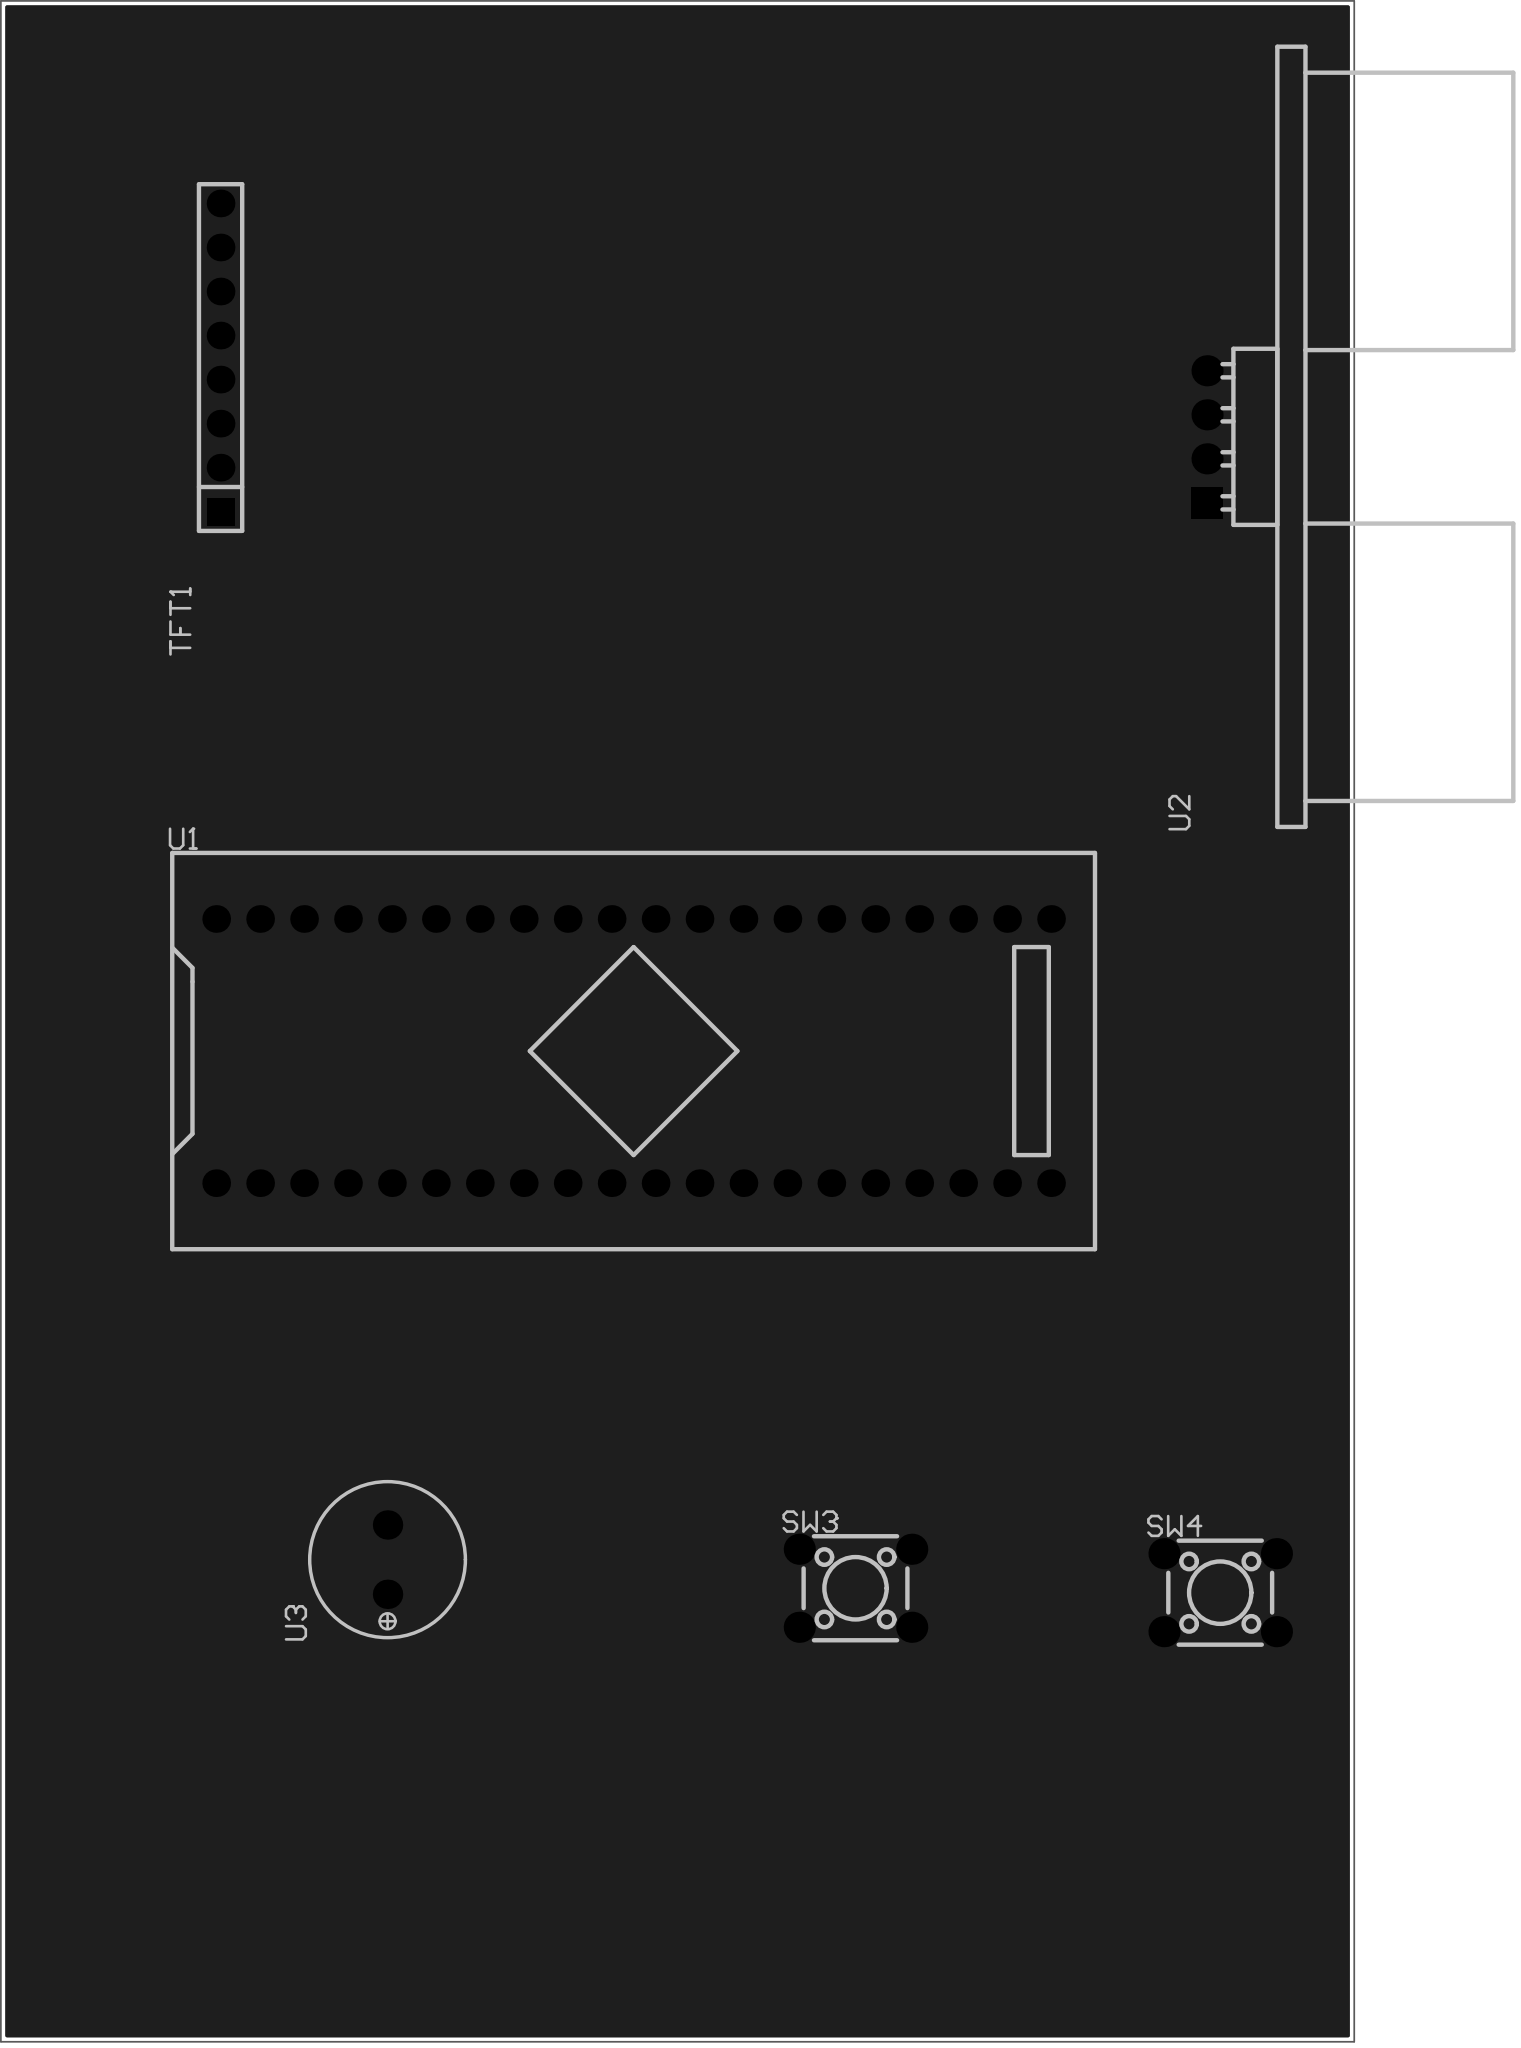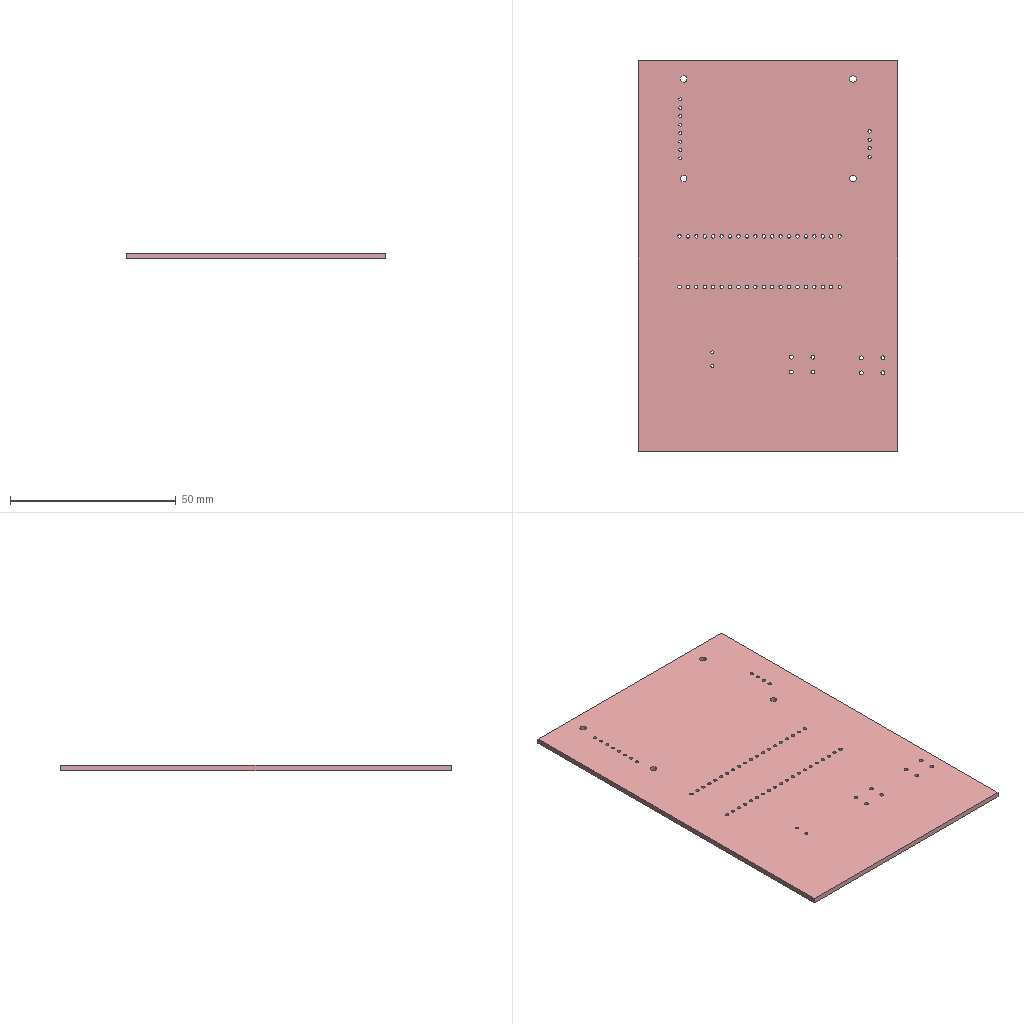Circuit board layout | Altium Designer | box 78.2 x 117.7 x 1.6 mm
Layer stack:
# Altium Designer layer stack of  (unit mm; dielectric type: 0 none, 1 core, 2 prepreg, 3 surface material)
index,name,kind,layer,copper_thickness_mm,dielectric_type,dielectric_thickness_mm,dielectric_material,dielectric_constant
0,Top Paste Mask Layer,other,,,,,,
1,Top Silkscreen Layer,other,,,,,,
2,Top Solder Mask Layer,dielectric,,,3,0.01,,3.3
3,Top Layer,copper,Top Layer,0.035,,,,
4,Dielectric1,dielectric,,,3,1.51,FR4,4.5
5,Bottom Layer,copper,Bottom Layer,0.035,,,,
6,Bottom Solder Mask Layer,dielectric,,,3,0.01,,3.3
7,Bottom Silkscreen Layer,other,,,,,,
8,Bottom Paste Mask Layer,other,,,,,,
# drill layer pairs: low layer,high layer
drill_pair,Top Layer,Bottom Layer
Part placement:
Designator,Comment,Layer,Footprint,Center-X(mm),Center-Y(mm),Rotation
TFT1,1.8 TFT 128*RGB*160,TopLayer,LCD-TH_8P-P2.54-L56.0-W34.0_1.8-TFT,111.125,209.296,90
SW3,,TopLayer,SW-TH_4P-L6.0-W6.0-P4.50-LS6.5,147.828,138.303,0
SW4,,TopLayer,SW-TH_4P-L6.0-W6.0-P4.50-LS6.5,168.91,138.049,0
U1,STM32F103C8T6-Card,TopLayer,CONN-TH_L53.3-W22.9_STM32F103C8T6-CARD,135.001,169.291,0
U2,HC-SR04,TopLayer,TH_HC-SR04V,168.148,204.724,90
U3,CUI_CST-931AP,TopLayer,BUZ-TH_BD9.0-P4.00-D0.6-L-FD,120.777,139.954,90
Pad and via stacks:
# Altium Designer via and pad stacks of  (unit mm). Each distinct definition once, with the count of objects using it.
# via: kind,start_layer,end_layer,hole_mm,diameter_mm,mode(0 simple;1 top-mid-bottom;2 full stack),diameter_per_layer,count,example_net
# pad: kind,layer,hole_mm,hole_type(0 round;1 square;2 slot),plating,top_size,top_shape(1 round;2 rect;3 octagon;9 rounded rect),mid_size,bottom_size,mode,footprint,size_per_layer,count,example
pad,Multi-Layer,0.9144,0,plated,1.6x1.6,2,1.6x1.6,1.6x1.6,0,LCD-TH_8P-P2.54-L56.0-W34.0_1.8-TFT,,1,TFT1.1
pad,Multi-Layer,0.9144,0,plated,1.6x1.6,1,1.6x1.6,1.6x1.6,0,LCD-TH_8P-P2.54-L56.0-W34.0_1.8-TFT,,7,TFT1.2
pad,Multi-Layer,1.2,0,plated,1.8x1.8,1,1.8x1.8,1.8x1.8,0,SW-TH_4P-L6.0-W6.0-P4.50-LS6.5,,8,SW3.1
pad,Multi-Layer,1,0,plated,1.6x1.6,1,1.6x1.6,1.6x1.6,0,CONN-TH_L53.3-W22.9_STM32F103C8T6-CARD,,40,U1.1
pad,Multi-Layer,1.001,0,plated,1.8x1.8,1,1.8x1.8,1.8x1.8,0,TH_HC-SR04V,,3,U2.4
pad,Multi-Layer,1.001,0,plated,1.8x1.8,2,1.8x1.8,1.8x1.8,0,TH_HC-SR04V,,1,U2.1
pad,Multi-Layer,0.9,0,plated,1.7x1.7,1,1.7x1.7,1.7x1.7,0,BUZ-TH_BD9.0-P4.00-D0.6-L-FD,,2,U3.2
Copper pours:
name,layer,net,type(0 solid;1 hatched;2 none)
Bottom Layer-GND,Bottom Layer,GND,0
Top Layer-GND,Top Layer,GND,0
Design rules, without the lines most boards share:
# Altium Designer design rules of  (exported by Altium Designer, unit mm)
# columns: name | kind | enabled | priority | scope1 | scope2 | descriptor | typed fields (field=value)
Copper_copperRegion_copperThickness1oz | 0 | disabled | 4 | All | All | Clearance Constraint (Gap=5.984mil) (Disabled)(All),(All) | gap=0.152
Copper_copperRegion_copperThickness1oz_1 | 63 | disabled | 4 | All | All | Board Clearance Constraint (Gap=0mil) (Disabled)(All) |
Copper_copperRegion_Copper_copperRegion | 0 | disabled | 5 | All | All | Clearance Constraint (Gap=5.984mil) (Disabled)(All),(All) | gap=0.152
Copper_copperRegion_Copper_copperRegion_1 | 63 | disabled | 5 | All | All | Board Clearance Constraint (Gap=0mil) (Disabled)(All) |
copperThickness1oz | 0 | enabled | 6 | All | All | Clearance Constraint (Gap=5.984mil) (All),(All) | gap=0.152
copperThickness1oz_1 | 63 | enabled | 6 | All | All | Board Clearance Constraint (Gap=0mil) (All) |
copperRegion_copperThickness1oz | 20 | enabled | 1 | (InNet('GND')) | All | Polygon Connect Rule(Relief Connect )(Conductor Width=10mil) (Relief Angle=90 Angle) (Entries=4) (Air Gap Width=10mil) ((InNet('GND'))),(All) | connect_style(0=relief,1=direct,2=none)=0 relief_conductor_width=0.254 relief_entries=4
copperRegion_Copper_copperRegion | 20 | disabled | 2 | All | All | Polygon Connect Rule(Relief Connect )(Conductor Width=10mil) (Relief Angle=90 Angle) (Entries=4) (Air Gap Width=10mil) (Disabled)(All),(All) | connect_style(0=relief,1=direct,2=none)=0 relief_conductor_width=0.254 relief_entries=4
copperRegion | 20 | enabled | 3 | All | All | Polygon Connect Rule(Relief Connect )(Conductor Width=10mil) (Relief Angle=90 Angle) (Entries=4) (Air Gap Width=10mil) (All),(All) | connect_style(0=relief,1=direct,2=none)=0 relief_conductor_width=0.254 relief_entries=4